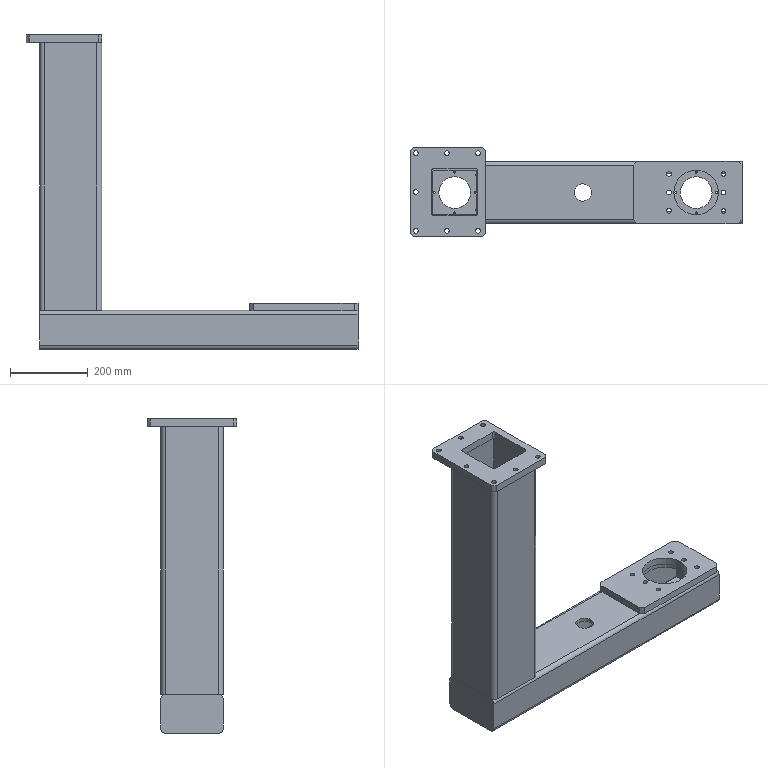Part | SolidWorks | features ICE 7, HoleWzd 4, Cut 3, Fillet 3, Chamfer 2, CirPattern 2, WeldMemberFeat 2, LPattern 1, WeldCornerFeat 1, WeldmentFeature 1 | 4 solids | 192 faces | box 855 x 230 x 810 mm | volume 8405482 mm3 | cylinder 130 | plane 62 | commonest cylinder face diameters 12 x58 3.3 x28 5 x16 1.572 x4 4.785 x4 21.572 x4